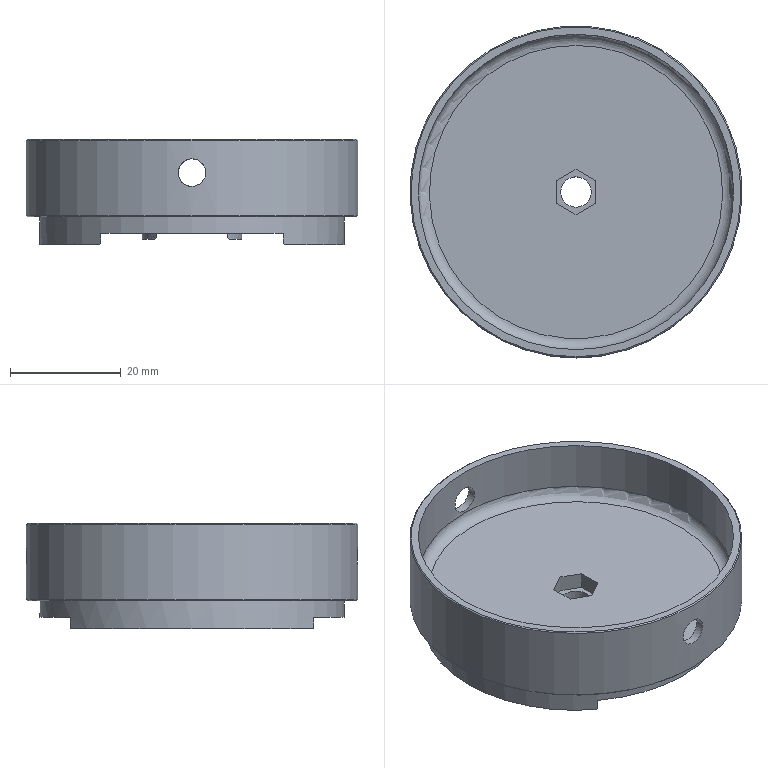NC program | NX | posted with a generic post | part box 60 x 60 x 19 mm
Lines 297 to 1274 of 13134:
(FLOOR_WALL_1_COPY_1 , TOOL : D17R0.8)
N586 T19 M6
N588 G54
N590 G17 G0 G90 X6.259 Y-4.944 S2000 M3
N592 G43 Z30. H19
N594 Z1.5
N596 G94 G1 X6.836 Y-4.214 Z1.451 F1000.
N598 X7.624 Y-2.522 Z1.353
N600 X8. Y-0.693 Z1.256
N602 Y0.693 Z1.183
N604 X7.624 Y2.522 Z1.085
N606 X6.836 Y4.214 Z0.987
N608 X5.678 Y5.678 Z0.889
N610 X4.214 Y6.836 Z0.792
N612 X2.522 Y7.624 Z0.694
N614 X0.693 Y8. Z0.596
N616 X-0.693 Z0.523
N618 X-2.522 Y7.624 Z0.425
N620 X-4.214 Y6.836 Z0.328
N622 X-5.678 Y5.678 Z0.23
N624 X-6.836 Y4.214 Z0.132
N626 X-7.624 Y2.522 Z0.034
N628 X-8. Y0.693 Z-0.064
N630 Y0. Z-0.1
N632 X-0.35
N634 G3 X0. Y-0.35 R0.35 F2000.
N636 X-0.35 Y0. R-0.35
N638 G1 X-8.
N640 G3 X0. Y-8. R8.
N642 X-8. Y0. R-8.
N644 G1 X-19.9
N646 G3 X0. Y-19.9 R19.9
N648 X-19.9 Y0. R-19.9
N650 G1 Z1.4
N652 G0 X-6.259 Y4.944
N654 G1 X-6.836 Y4.214 Z1.351 F1000.
N656 X-7.624 Y2.522 Z1.253
N658 X-8. Y0.693 Z1.156
N660 Y-0.693 Z1.083
N662 X-7.624 Y-2.522 Z0.985
N664 X-6.836 Y-4.214 Z0.887
N666 X-5.678 Y-5.678 Z0.789
N668 X-4.214 Y-6.836 Z0.692
N670 X-2.522 Y-7.624 Z0.594
N672 X-0.693 Y-8. Z0.496
N674 X0.693 Z0.423
N676 X2.522 Y-7.624 Z0.325
N678 X4.214 Y-6.836 Z0.228
N680 X5.678 Y-5.678 Z0.13
N682 X6.836 Y-4.214 Z0.032
N684 X7.624 Y-2.522 Z-0.066
N686 X8. Y-0.693 Z-0.164
N688 Y0. Z-0.2
N690 X0.35
N692 G3 X0. Y0.35 R0.35 F2000.
N694 X0.35 Y0. R-0.35
N696 G1 X8.
N698 G3 X0. Y8. R8.
N700 X8. Y0. R-8.
N702 G1 X19.9
N704 G3 X0. Y19.9 R19.9
N706 X19.9 Y0. R-19.9
N708 G1 Z1.3
N710 G0 X-6.259 Y4.944
N712 G1 X-6.836 Y4.214 Z1.251 F1000.
N714 X-7.624 Y2.522 Z1.153
N716 X-8. Y0.693 Z1.056
N718 Y-0.693 Z0.983
N720 X-7.624 Y-2.522 Z0.885
N722 X-6.836 Y-4.214 Z0.787
N724 X-5.678 Y-5.678 Z0.689
N726 X-4.214 Y-6.836 Z0.592
N728 X-2.522 Y-7.624 Z0.494
N730 X-0.693 Y-8. Z0.396
N732 X0.693 Z0.323
N734 X2.522 Y-7.624 Z0.225
N736 X4.214 Y-6.836 Z0.128
N738 X5.678 Y-5.678 Z0.03
N740 X6.836 Y-4.214 Z-0.068
N742 X7.624 Y-2.522 Z-0.166
N744 X8. Y-0.693 Z-0.264
N746 Y0. Z-0.3
N748 X0.35
N750 G3 X0. Y0.35 R0.35 F2000.
N752 X0.35 Y0. R-0.35
N754 G1 X8.
N756 G3 X0. Y8. R8.
N758 X8. Y0. R-8.
N760 G1 X19.9
N762 G3 X0. Y19.9 R19.9
N764 X19.9 Y0. R-19.9
N766 G1 Z1.2
N768 G0 X-6.259 Y4.944
N770 G1 X-6.836 Y4.214 Z1.151 F1000.
N772 X-7.624 Y2.522 Z1.053
N774 X-8. Y0.693 Z0.956
N776 Y-0.693 Z0.883
N778 X-7.624 Y-2.522 Z0.785
N780 X-6.836 Y-4.214 Z0.687
N782 X-5.678 Y-5.678 Z0.589
N784 X-4.214 Y-6.836 Z0.492
N786 X-2.522 Y-7.624 Z0.394
N788 X-0.693 Y-8. Z0.296
N790 X0.693 Z0.223
N792 X2.522 Y-7.624 Z0.125
N794 X4.214 Y-6.836 Z0.028
N796 X5.678 Y-5.678 Z-0.07
N798 X6.836 Y-4.214 Z-0.168
N800 X7.624 Y-2.522 Z-0.266
N802 X8. Y-0.693 Z-0.364
N804 Y0. Z-0.4
N806 X0.35
N808 G3 X0. Y0.35 R0.35 F2000.
N810 X0.35 Y0. R-0.35
N812 G1 X8.
N814 G3 X0. Y8. R8.
N816 X8. Y0. R-8.
N818 G1 X19.9
N820 G3 X0. Y19.9 R19.9
N822 X19.9 Y0. R-19.9
N824 G1 Z1.1
N826 G0 X-6.259 Y4.944
N828 G1 X-6.836 Y4.214 Z1.051 F1000.
N830 X-7.624 Y2.522 Z0.953
N832 X-8. Y0.693 Z0.856
N834 Y-0.693 Z0.783
N836 X-7.624 Y-2.522 Z0.685
N838 X-6.836 Y-4.214 Z0.587
N840 X-5.678 Y-5.678 Z0.489
N842 X-4.214 Y-6.836 Z0.392
N844 X-2.522 Y-7.624 Z0.294
N846 X-0.693 Y-8. Z0.196
N848 X0.693 Z0.123
N850 X2.522 Y-7.624 Z0.025
N852 X4.214 Y-6.836 Z-0.072
N854 X5.678 Y-5.678 Z-0.17
N856 X6.836 Y-4.214 Z-0.268
N858 X7.624 Y-2.522 Z-0.366
N860 X8. Y-0.693 Z-0.464
N862 Y0. Z-0.5
N864 X0.35
N866 G3 X0. Y0.35 R0.35 F2000.
N868 X0.35 Y0. R-0.35
N870 G1 X8.
N872 G3 X0. Y8. R8.
N874 X8. Y0. R-8.
N876 G1 X19.9
N878 G3 X0. Y19.9 R19.9
N880 X19.9 Y0. R-19.9
N882 G1 Z1.
N884 G0 X-6.259 Y4.944
N886 G1 X-6.836 Y4.214 Z0.951 F1000.
N888 X-7.624 Y2.522 Z0.853
N890 X-8. Y0.693 Z0.756
N892 Y-0.693 Z0.683
N894 X-7.624 Y-2.522 Z0.585
N896 X-6.836 Y-4.214 Z0.487
N898 X-5.678 Y-5.678 Z0.389
N900 X-4.214 Y-6.836 Z0.292
N902 X-2.522 Y-7.624 Z0.194
N904 X-0.693 Y-8. Z0.096
N906 X0.693 Z0.023
N908 X2.522 Y-7.624 Z-0.075
N910 X4.214 Y-6.836 Z-0.172
N912 X5.678 Y-5.678 Z-0.27
N914 X6.836 Y-4.214 Z-0.368
N916 X7.624 Y-2.522 Z-0.466
N918 X8. Y-0.693 Z-0.564
N920 Y0. Z-0.6
N922 X0.35
N924 G3 X0. Y0.35 R0.35 F2000.
N926 X0.35 Y0. R-0.35
N928 G1 X8.
N930 G3 X0. Y8. R8.
N932 X8. Y0. R-8.
N934 G1 X19.9
N936 G3 X0. Y19.9 R19.9
N938 X19.9 Y0. R-19.9
N940 G1 Z0.9
N942 G0 X-6.259 Y4.944
N944 G1 X-6.836 Y4.214 Z0.851 F1000.
N946 X-7.624 Y2.522 Z0.753
N948 X-8. Y0.693 Z0.656
N950 Y-0.693 Z0.583
N952 X-7.624 Y-2.522 Z0.485
N954 X-6.836 Y-4.214 Z0.387
N956 X-5.678 Y-5.678 Z0.289
N958 X-4.214 Y-6.836 Z0.192
N960 X-2.522 Y-7.624 Z0.094
N962 X-0.693 Y-8. Z-0.004
N964 X0.693 Z-0.077
N966 X2.522 Y-7.624 Z-0.175
N968 X4.214 Y-6.836 Z-0.272
N970 X5.678 Y-5.678 Z-0.37
N972 X6.836 Y-4.214 Z-0.468
N974 X7.624 Y-2.522 Z-0.566
N976 X8. Y-0.693 Z-0.664
N978 Y0. Z-0.7
N980 X0.35
N982 G3 X0. Y0.35 R0.35 F2000.
N984 X0.35 Y0. R-0.35
N986 G1 X8.
N988 G3 X0. Y8. R8.
N990 X8. Y0. R-8.
N992 G1 X19.9
N994 G3 X0. Y19.9 R19.9
N996 X19.9 Y0. R-19.9
N998 G1 Z0.8
N1000 G0 X-6.259 Y4.944
N1002 G1 X-6.836 Y4.214 Z0.751 F1000.
N1004 X-7.624 Y2.522 Z0.653
N1006 X-8. Y0.693 Z0.556
N1008 Y-0.693 Z0.483
N1010 X-7.624 Y-2.522 Z0.385
N1012 X-6.836 Y-4.214 Z0.287
N1014 X-5.678 Y-5.678 Z0.189
N1016 X-4.214 Y-6.836 Z0.092
N1018 X-2.522 Y-7.624 Z-0.006
N1020 X-0.693 Y-8. Z-0.104
N1022 X0.693 Z-0.177
N1024 X2.522 Y-7.624 Z-0.275
N1026 X4.214 Y-6.836 Z-0.372
N1028 X5.678 Y-5.678 Z-0.47
N1030 X6.836 Y-4.214 Z-0.568
N1032 X7.624 Y-2.522 Z-0.666
N1034 X8. Y-0.693 Z-0.764
N1036 Y0. Z-0.8
N1038 X0.35
N1040 G3 X0. Y0.35 R0.35 F2000.
N1042 X0.35 Y0. R-0.35
N1044 G1 X8.
N1046 G3 X0. Y8. R8.
N1048 X8. Y0. R-8.
N1050 G1 X19.9
N1052 G3 X0. Y19.9 R19.9
N1054 X19.9 Y0. R-19.9
N1056 G1 Z0.7
N1058 G0 X-6.259 Y4.944
N1060 G1 X-6.836 Y4.214 Z0.651 F1000.
N1062 X-7.624 Y2.522 Z0.553
N1064 X-8. Y0.693 Z0.456
N1066 Y-0.693 Z0.383
N1068 X-7.624 Y-2.522 Z0.285
N1070 X-6.836 Y-4.214 Z0.187
N1072 X-5.678 Y-5.678 Z0.089
N1074 X-4.214 Y-6.836 Z-0.008
N1076 X-2.522 Y-7.624 Z-0.106
N1078 X-0.693 Y-8. Z-0.204
N1080 X0.693 Z-0.277
N1082 X2.522 Y-7.624 Z-0.375
N1084 X4.214 Y-6.836 Z-0.472
N1086 X5.678 Y-5.678 Z-0.57
N1088 X6.836 Y-4.214 Z-0.668
N1090 X7.624 Y-2.522 Z-0.766
N1092 X8. Y-0.693 Z-0.864
N1094 Y0. Z-0.9
N1096 X0.35
N1098 G3 X0. Y0.35 R0.35 F2000.
N1100 X0.35 Y0. R-0.35
N1102 G1 X8.
N1104 G3 X0. Y8. R8.
N1106 X8. Y0. R-8.
N1108 G1 X19.9
N1110 G3 X0. Y19.9 R19.9
N1112 X19.9 Y0. R-19.9
N1114 G1 Z0.6
N1116 G0 X-6.259 Y4.944
N1118 G1 X-6.836 Y4.214 Z0.551 F1000.
N1120 X-7.624 Y2.522 Z0.453
N1122 X-8. Y0.693 Z0.356
N1124 Y-0.693 Z0.283
N1126 X-7.624 Y-2.522 Z0.185
N1128 X-6.836 Y-4.214 Z0.087
N1130 X-5.678 Y-5.678 Z-0.011
N1132 X-4.214 Y-6.836 Z-0.108
N1134 X-2.522 Y-7.624 Z-0.206
N1136 X-0.693 Y-8. Z-0.304
N1138 X0.693 Z-0.377
N1140 X2.522 Y-7.624 Z-0.475
N1142 X4.214 Y-6.836 Z-0.572
N1144 X5.678 Y-5.678 Z-0.67
N1146 X6.836 Y-4.214 Z-0.768
N1148 X7.624 Y-2.522 Z-0.866
N1150 X8. Y-0.693 Z-0.964
N1152 Y0. Z-1.
N1154 X0.35
N1156 G3 X0. Y0.35 R0.35 F2000.
N1158 X0.35 Y0. R-0.35
N1160 G1 X8.
N1162 G3 X0. Y8. R8.
N1164 X8. Y0. R-8.
N1166 G1 X19.9
N1168 G3 X0. Y19.9 R19.9
N1170 X19.9 Y0. R-19.9
N1172 G1 Z0.5
N1174 G0 X-6.259 Y4.944
N1176 G1 X-6.836 Y4.214 Z0.451 F1000.
N1178 X-7.624 Y2.522 Z0.353
N1180 X-8. Y0.693 Z0.256
N1182 Y-0.693 Z0.183
N1184 X-7.624 Y-2.522 Z0.085
N1186 X-6.836 Y-4.214 Z-0.013
N1188 X-5.678 Y-5.678 Z-0.111
N1190 X-4.214 Y-6.836 Z-0.208
N1192 X-2.522 Y-7.624 Z-0.306
N1194 X-0.693 Y-8. Z-0.404
N1196 X0.693 Z-0.477
N1198 X2.522 Y-7.624 Z-0.575
N1200 X4.214 Y-6.836 Z-0.672
N1202 X5.678 Y-5.678 Z-0.77
N1204 X6.836 Y-4.214 Z-0.868
N1206 X7.624 Y-2.522 Z-0.966
N1208 X8. Y-0.693 Z-1.064
N1210 Y0. Z-1.1
N1212 X0.35
N1214 G3 X0. Y0.35 R0.35 F2000.
N1216 X0.35 Y0. R-0.35
N1218 G1 X8.
N1220 G3 X0. Y8. R8.
N1222 X8. Y0. R-8.
N1224 G1 X19.9
N1226 G3 X0. Y19.9 R19.9
N1228 X19.9 Y0. R-19.9
N1230 G1 Z0.4
N1232 G0 X-6.259 Y4.944
N1234 G1 X-6.836 Y4.214 Z0.351 F1000.
N1236 X-7.624 Y2.522 Z0.253
N1238 X-8. Y0.693 Z0.156
N1240 Y-0.693 Z0.083
N1242 X-7.624 Y-2.522 Z-0.015
N1244 X-6.836 Y-4.214 Z-0.113
N1246 X-5.678 Y-5.678 Z-0.211
N1248 X-4.214 Y-6.836 Z-0.308
N1250 X-2.522 Y-7.624 Z-0.406
N1252 X-0.693 Y-8. Z-0.504
N1254 X0.693 Z-0.577
N1256 X2.522 Y-7.624 Z-0.675
N1258 X4.214 Y-6.836 Z-0.772
N1260 X5.678 Y-5.678 Z-0.87
N1262 X6.836 Y-4.214 Z-0.968
N1264 X7.624 Y-2.522 Z-1.066
N1266 X8. Y-0.693 Z-1.164
N1268 Y0. Z-1.2
N1270 X0.35
N1272 G3 X0. Y0.35 R0.35 F2000.
N1274 X0.35 Y0. R-0.35
N1276 G1 X8.
N1278 G3 X0. Y8. R8.
N1280 X8. Y0. R-8.
N1282 G1 X19.9
N1284 G3 X0. Y19.9 R19.9
N1286 X19.9 Y0. R-19.9
N1288 G1 Z0.3
N1290 G0 X-6.259 Y4.944
N1292 G1 X-6.836 Y4.214 Z0.251 F1000.
N1294 X-7.624 Y2.522 Z0.153
N1296 X-8. Y0.693 Z0.056
N1298 Y-0.693 Z-0.017
N1300 X-7.624 Y-2.522 Z-0.115
N1302 X-6.836 Y-4.214 Z-0.213
N1304 X-5.678 Y-5.678 Z-0.311
N1306 X-4.214 Y-6.836 Z-0.408
N1308 X-2.522 Y-7.624 Z-0.506
N1310 X-0.693 Y-8. Z-0.604
N1312 X0.693 Z-0.677
N1314 X2.522 Y-7.624 Z-0.775
N1316 X4.214 Y-6.836 Z-0.872
N1318 X5.678 Y-5.678 Z-0.97
N1320 X6.836 Y-4.214 Z-1.068
N1322 X7.624 Y-2.522 Z-1.166
N1324 X8. Y-0.693 Z-1.264
N1326 Y0. Z-1.3
N1328 X0.35
N1330 G3 X0. Y0.35 R0.35 F2000.
N1332 X0.35 Y0. R-0.35
N1334 G1 X8.
N1336 G3 X0. Y8. R8.
N1338 X8. Y0. R-8.
N1340 G1 X19.9
N1342 G3 X0. Y19.9 R19.9
N1344 X19.9 Y0. R-19.9
N1346 G1 Z0.2
N1348 G0 X-6.259 Y4.944
N1350 G1 X-6.836 Y4.214 Z0.151 F1000.
N1352 X-7.624 Y2.522 Z0.053
N1354 X-8. Y0.693 Z-0.044
N1356 Y-0.693 Z-0.117
N1358 X-7.624 Y-2.522 Z-0.215
N1360 X-6.836 Y-4.214 Z-0.313
N1362 X-5.678 Y-5.678 Z-0.411
N1364 X-4.214 Y-6.836 Z-0.508
N1366 X-2.522 Y-7.624 Z-0.606
N1368 X-0.693 Y-8. Z-0.704
N1370 X0.693 Z-0.777
N1372 X2.522 Y-7.624 Z-0.875
N1374 X4.214 Y-6.836 Z-0.972
N1376 X5.678 Y-5.678 Z-1.07
N1378 X6.836 Y-4.214 Z-1.168
N1380 X7.624 Y-2.522 Z-1.266
N1382 X8. Y-0.693 Z-1.364
N1384 Y0. Z-1.4
N1386 X0.35
N1388 G3 X0. Y0.35 R0.35 F2000.
N1390 X0.35 Y0. R-0.35
N1392 G1 X8.
N1394 G3 X0. Y8. R8.
N1396 X8. Y0. R-8.
N1398 G1 X19.9
N1400 G3 X0. Y19.9 R19.9
N1402 X19.9 Y0. R-19.9
N1404 G1 Z0.1
N1406 G0 X-6.259 Y4.944
N1408 G1 X-6.836 Y4.214 Z0.051 F1000.
N1410 X-7.624 Y2.522 Z-0.047
N1412 X-8. Y0.693 Z-0.144
N1414 Y-0.693 Z-0.217
N1416 X-7.624 Y-2.522 Z-0.315
N1418 X-6.836 Y-4.214 Z-0.413
N1420 X-5.678 Y-5.678 Z-0.511
N1422 X-4.214 Y-6.836 Z-0.608
N1424 X-2.522 Y-7.624 Z-0.706
N1426 X-0.693 Y-8. Z-0.804
N1428 X0.693 Z-0.877
N1430 X2.522 Y-7.624 Z-0.975
N1432 X4.214 Y-6.836 Z-1.072
N1434 X5.678 Y-5.678 Z-1.17
N1436 X6.836 Y-4.214 Z-1.268
N1438 X7.624 Y-2.522 Z-1.366
N1440 X8. Y-0.693 Z-1.464
N1442 Y0. Z-1.5
N1444 X0.35
N1446 G3 X0. Y0.35 R0.35 F2000.
N1448 X0.35 Y0. R-0.35
N1450 G1 X8.
N1452 G3 X0. Y8. R8.
N1454 X8. Y0. R-8.
N1456 G1 X19.9
N1458 G3 X0. Y19.9 R19.9
N1460 X19.9 Y0. R-19.9
N1462 G1 Z0.
N1464 G0 X-6.259 Y4.944
N1466 G1 X-6.836 Y4.214 Z-0.049 F1000.
N1468 X-7.624 Y2.522 Z-0.147
N1470 X-8. Y0.693 Z-0.244
N1472 Y-0.693 Z-0.317
N1474 X-7.624 Y-2.522 Z-0.415
N1476 X-6.836 Y-4.214 Z-0.513
N1478 X-5.678 Y-5.678 Z-0.611
N1480 X-4.214 Y-6.836 Z-0.708
N1482 X-2.522 Y-7.624 Z-0.806
N1484 X-0.693 Y-8. Z-0.904
N1486 X0.693 Z-0.977
N1488 X2.522 Y-7.624 Z-1.075
N1490 X4.214 Y-6.836 Z-1.172
N1492 X5.678 Y-5.678 Z-1.27
N1494 X6.836 Y-4.214 Z-1.368
N1496 X7.624 Y-2.522 Z-1.466
N1498 X8. Y-0.693 Z-1.564
N1500 Y0. Z-1.6
N1502 X0.35
N1504 G3 X0. Y0.35 R0.35 F2000.
N1506 X0.35 Y0. R-0.35
N1508 G1 X8.
N1510 G3 X0. Y8. R8.
N1512 X8. Y0. R-8.
N1514 G1 X19.9
N1516 G3 X0. Y19.9 R19.9
N1518 X19.9 Y0. R-19.9
N1520 G1 Z-0.1
N1522 G0 X-6.259 Y4.944
N1524 G1 X-6.836 Y4.214 Z-0.149 F1000.
N1526 X-7.624 Y2.522 Z-0.247
N1528 X-8. Y0.693 Z-0.344
N1530 Y-0.693 Z-0.417
N1532 X-7.624 Y-2.522 Z-0.515
N1534 X-6.836 Y-4.214 Z-0.613
N1536 X-5.678 Y-5.678 Z-0.711
N1538 X-4.214 Y-6.836 Z-0.808
N1540 X-2.522 Y-7.624 Z-0.906
N1542 X-0.693 Y-8. Z-1.004
N1544 X0.693 Z-1.077
N1546 X2.522 Y-7.624 Z-1.175
N1548 X4.214 Y-6.836 Z-1.272
N1550 X5.678 Y-5.678 Z-1.37
N1552 X6.836 Y-4.214 Z-1.468
N1554 X7.624 Y-2.522 Z-1.566
N1556 X8. Y-0.693 Z-1.664
N1558 Y0. Z-1.7
N1560 X0.35
N1562 G3 X0. Y0.35 R0.35 F2000.
N1564 X0.35 Y0. R-0.35
N1566 G1 X8.
N1568 G3 X0. Y8. R8.
N1570 X8. Y0. R-8.
N1572 G1 X19.9
N1574 G3 X0. Y19.9 R19.9
N1576 X19.9 Y0. R-19.9
N1578 G1 Z-0.2
N1580 G0 X-6.259 Y4.944
N1582 G1 X-6.836 Y4.214 Z-0.249 F1000.
N1584 X-7.624 Y2.522 Z-0.347
N1586 X-8. Y0.693 Z-0.444
N1588 Y-0.693 Z-0.517
N1590 X-7.624 Y-2.522 Z-0.615
N1592 X-6.836 Y-4.214 Z-0.713
N1594 X-5.678 Y-5.678 Z-0.811
N1596 X-4.214 Y-6.836 Z-0.908
N1598 X-2.522 Y-7.624 Z-1.006
N1600 X-0.693 Y-8. Z-1.104
N1602 X0.693 Z-1.177
N1604 X2.522 Y-7.624 Z-1.275
N1606 X4.214 Y-6.836 Z-1.372
N1608 X5.678 Y-5.678 Z-1.47
N1610 X6.836 Y-4.214 Z-1.568
N1612 X7.624 Y-2.522 Z-1.666
N1614 X8. Y-0.693 Z-1.764
N1616 Y0. Z-1.8
N1618 X0.35
N1620 G3 X0. Y0.35 R0.35 F2000.
N1622 X0.35 Y0. R-0.35
N1624 G1 X8.
N1626 G3 X0. Y8. R8.
N1628 X8. Y0. R-8.
N1630 G1 X19.9
N1632 G3 X0. Y19.9 R19.9
N1634 X19.9 Y0. R-19.9
N1636 G1 Z-0.3
N1638 G0 X-6.259 Y4.944
N1640 G1 X-6.836 Y4.214 Z-0.349 F1000.
N1642 X-7.624 Y2.522 Z-0.447
N1644 X-8. Y0.693 Z-0.544
N1646 Y-0.693 Z-0.617
N1648 X-7.624 Y-2.522 Z-0.715
N1650 X-6.836 Y-4.214 Z-0.813
N1652 X-5.678 Y-5.678 Z-0.911
N1654 X-4.214 Y-6.836 Z-1.008
N1656 X-2.522 Y-7.624 Z-1.106
N1658 X-0.693 Y-8. Z-1.204
N1660 X0.693 Z-1.277
N1662 X2.522 Y-7.624 Z-1.375
N1664 X4.214 Y-6.836 Z-1.472
N1666 X5.678 Y-5.678 Z-1.57
N1668 X6.836 Y-4.214 Z-1.668
N1670 X7.624 Y-2.522 Z-1.766
N1672 X8. Y-0.693 Z-1.864
N1674 Y0. Z-1.9
N1676 X0.35
N1678 G3 X0. Y0.35 R0.35 F2000.
N1680 X0.35 Y0. R-0.35
N1682 G1 X8.
N1684 G3 X0. Y8. R8.
N1686 X8. Y0. R-8.
N1688 G1 X19.9
N1690 G3 X0. Y19.9 R19.9
N1692 X19.9 Y0. R-19.9
N1694 G1 Z-0.4
N1696 G0 X-6.259 Y4.944
N1698 G1 X-6.836 Y4.214 Z-0.449 F1000.
N1700 X-7.624 Y2.522 Z-0.547
N1702 X-8. Y0.693 Z-0.644
N1704 Y-0.693 Z-0.717
N1706 X-7.624 Y-2.522 Z-0.815
N1708 X-6.836 Y-4.214 Z-0.913
N1710 X-5.678 Y-5.678 Z-1.011
N1712 X-4.214 Y-6.836 Z-1.108
N1714 X-2.522 Y-7.624 Z-1.206
N1716 X-0.693 Y-8. Z-1.304
N1718 X0.693 Z-1.377
N1720 X2.522 Y-7.624 Z-1.475
N1722 X4.214 Y-6.836 Z-1.572
N1724 X5.678 Y-5.678 Z-1.67
N1726 X6.836 Y-4.214 Z-1.768
N1728 X7.624 Y-2.522 Z-1.866
N1730 X8. Y-0.693 Z-1.964
N1732 Y0. Z-2.
N1734 X0.35
N1736 G3 X0. Y0.35 R0.35 F2000.
N1738 X0.35 Y0. R-0.35
N1740 G1 X8.
N1742 G3 X0. Y8. R8.
N1744 X8. Y0. R-8.
N1746 G1 X19.9
N1748 G3 X0. Y19.9 R19.9
N1750 X19.9 Y0. R-19.9
N1752 G1 Z-0.5
N1754 G0 X-6.259 Y4.944
N1756 G1 X-6.836 Y4.214 Z-0.549 F1000.
N1758 X-7.624 Y2.522 Z-0.647
N1760 X-8. Y0.693 Z-0.744
N1762 Y-0.693 Z-0.817
N1764 X-7.624 Y-2.522 Z-0.915
N1766 X-6.836 Y-4.214 Z-1.013
N1768 X-5.678 Y-5.678 Z-1.111
N1770 X-4.214 Y-6.836 Z-1.208
N1772 X-2.522 Y-7.624 Z-1.306
N1774 X-0.693 Y-8. Z-1.404
N1776 X0.693 Z-1.477
N1778 X2.522 Y-7.624 Z-1.575
N1780 X4.214 Y-6.836 Z-1.672
N1782 X5.678 Y-5.678 Z-1.77
N1784 X6.836 Y-4.214 Z-1.868
N1786 X7.624 Y-2.522 Z-1.966
N1788 X8. Y-0.693 Z-2.064
N1790 Y0. Z-2.1
N1792 X0.35
N1794 G3 X0. Y0.35 R0.35 F2000.
N1796 X0.35 Y0. R-0.35
N1798 G1 X8.
N1800 G3 X0. Y8. R8.
N1802 X8. Y0. R-8.
N1804 G1 X19.9
N1806 G3 X0. Y19.9 R19.9
N1808 X19.9 Y0. R-19.9
N1810 G1 Z-0.6
N1812 G0 X-6.259 Y4.944
N1814 G1 X-6.836 Y4.214 Z-0.649 F1000.
N1816 X-7.624 Y2.522 Z-0.747
N1818 X-8. Y0.693 Z-0.844
N1820 Y-0.693 Z-0.917
N1822 X-7.624 Y-2.522 Z-1.015
N1824 X-6.836 Y-4.214 Z-1.113
N1826 X-5.678 Y-5.678 Z-1.211
N1828 X-4.214 Y-6.836 Z-1.308
N1830 X-2.522 Y-7.624 Z-1.406
N1832 X-0.693 Y-8. Z-1.504
N1834 X0.693 Z-1.577
N1836 X2.522 Y-7.624 Z-1.675
N1838 X4.214 Y-6.836 Z-1.772
N1840 X5.678 Y-5.678 Z-1.87
N1842 X6.836 Y-4.214 Z-1.968
N1844 X7.624 Y-2.522 Z-2.066
N1846 X8. Y-0.693 Z-2.164
N1848 Y0. Z-2.2
N1850 X0.35
N1852 G3 X0. Y0.35 R0.35 F2000.
N1854 X0.35 Y0. R-0.35
N1856 G1 X8.
N1858 G3 X0. Y8. R8.
N1860 X8. Y0. R-8.
N1862 G1 X19.9
N1864 G3 X0. Y19.9 R19.9
N1866 X19.9 Y0. R-19.9
N1868 G1 Z-0.7
N1870 G0 X-6.259 Y4.944
N1872 G1 X-6.836 Y4.214 Z-0.749 F1000.
N1874 X-7.624 Y2.522 Z-0.847
N1876 X-8. Y0.693 Z-0.944
N1878 Y-0.693 Z-1.017
N1880 X-7.624 Y-2.522 Z-1.115
N1882 X-6.836 Y-4.214 Z-1.213
N1884 X-5.678 Y-5.678 Z-1.311
N1886 X-4.214 Y-6.836 Z-1.408
N1888 X-2.522 Y-7.624 Z-1.506
N1890 X-0.693 Y-8. Z-1.604
N1892 X0.693 Z-1.677
N1894 X2.522 Y-7.624 Z-1.775
N1896 X4.214 Y-6.836 Z-1.872
N1898 X5.678 Y-5.678 Z-1.97
N1900 X6.836 Y-4.214 Z-2.068
N1902 X7.624 Y-2.522 Z-2.166
N1904 X8. Y-0.693 Z-2.264
N1906 Y0. Z-2.3
N1908 X0.35
N1910 G3 X0. Y0.35 R0.35 F2000.
N1912 X0.35 Y0. R-0.35
N1914 G1 X8.
N1916 G3 X0. Y8. R8.
N1918 X8. Y0. R-8.
N1920 G1 X19.9
N1922 G3 X0. Y19.9 R19.9
N1924 X19.9 Y0. R-19.9
N1926 G1 Z-0.8
N1928 G0 X-6.259 Y4.944
N1930 G1 X-6.836 Y4.214 Z-0.849 F1000.
N1932 X-7.624 Y2.522 Z-0.947
N1934 X-8. Y0.693 Z-1.044
N1936 Y-0.693 Z-1.117
N1938 X-7.624 Y-2.522 Z-1.215
N1940 X-6.836 Y-4.214 Z-1.313
N1942 X-5.678 Y-5.678 Z-1.411
N1944 X-4.214 Y-6.836 Z-1.508
N1946 X-2.522 Y-7.624 Z-1.606
N1948 X-0.693 Y-8. Z-1.704
N1950 X0.693 Z-1.777
N1952 X2.522 Y-7.624 Z-1.875
N1954 X4.214 Y-6.836 Z-1.972
N1956 X5.678 Y-5.678 Z-2.07
N1958 X6.836 Y-4.214 Z-2.168
N1960 X7.624 Y-2.522 Z-2.266
N1962 X8. Y-0.693 Z-2.364
N1964 Y0. Z-2.4
N1966 X0.35
N1968 G3 X0. Y0.35 R0.35 F2000.
N1970 X0.35 Y0. R-0.35
N1972 G1 X8.
N1974 G3 X0. Y8. R8.
N1976 X8. Y0. R-8.
N1978 G1 X19.9
N1980 G3 X0. Y19.9 R19.9
N1982 X19.9 Y0. R-19.9
N1984 G1 Z-0.9
N1986 G0 X-6.259 Y4.944
N1988 G1 X-6.836 Y4.214 Z-0.949 F1000.
N1990 X-7.624 Y2.522 Z-1.047
N1992 X-8. Y0.693 Z-1.144
N1994 Y-0.693 Z-1.217
N1996 X-7.624 Y-2.522 Z-1.315
N1998 X-6.836 Y-4.214 Z-1.413
N2000 X-5.678 Y-5.678 Z-1.511
N2002 X-4.214 Y-6.836 Z-1.608
N2004 X-2.522 Y-7.624 Z-1.706
N2006 X-0.693 Y-8. Z-1.804
N2008 X0.693 Z-1.877
N2010 X2.522 Y-7.624 Z-1.975
N2012 X4.214 Y-6.836 Z-2.072
N2014 X5.678 Y-5.678 Z-2.17
N2016 X6.836 Y-4.214 Z-2.268
N2018 X7.624 Y-2.522 Z-2.366
N2020 X8. Y-0.693 Z-2.464
N2022 Y0. Z-2.5
N2024 X0.35
N2026 G3 X0. Y0.35 R0.35 F2000.
N2028 X0.35 Y0. R-0.35
N2030 G1 X8.
N2032 G3 X0. Y8. R8.
N2034 X8. Y0. R-8.
N2036 G1 X19.9
N2038 G3 X0. Y19.9 R19.9
N2040 X19.9 Y0. R-19.9
N2042 G1 Z-1.
N2044 G0 X-6.259 Y4.944
N2046 G1 X-6.836 Y4.214 Z-1.049 F1000.
N2048 X-7.624 Y2.522 Z-1.147
N2050 X-8. Y0.693 Z-1.244
N2052 Y-0.693 Z-1.317
N2054 X-7.624 Y-2.522 Z-1.415
N2056 X-6.836 Y-4.214 Z-1.513
N2058 X-5.678 Y-5.678 Z-1.611
N2060 X-4.214 Y-6.836 Z-1.708
N2062 X-2.522 Y-7.624 Z-1.806
N2064 X-0.693 Y-8. Z-1.904
N2066 X0.693 Z-1.977
N2068 X2.522 Y-7.624 Z-2.075
N2070 X4.214 Y-6.836 Z-2.172
N2072 X5.678 Y-5.678 Z-2.27
N2074 X6.836 Y-4.214 Z-2.368
N2076 X7.624 Y-2.522 Z-2.466
N2078 X8. Y-0.693 Z-2.564
N2080 Y0. Z-2.6
N2082 X0.35
N2084 G3 X0. Y0.35 R0.35 F2000.
N2086 X0.35 Y0. R-0.35
N2088 G1 X8.
N2090 G3 X0. Y8. R8.
N2092 X8. Y0. R-8.
N2094 G1 X19.9
N2096 G3 X0. Y19.9 R19.9
N2098 X19.9 Y0. R-19.9
N2100 G1 Z-1.1
N2102 G0 X-6.259 Y4.944
N2104 G1 X-6.836 Y4.214 Z-1.149 F1000.
N2106 X-7.624 Y2.522 Z-1.247
N2108 X-8. Y0.693 Z-1.344
N2110 Y-0.693 Z-1.417
N2112 X-7.624 Y-2.522 Z-1.515
N2114 X-6.836 Y-4.214 Z-1.613
N2116 X-5.678 Y-5.678 Z-1.711
N2118 X-4.214 Y-6.836 Z-1.808
N2120 X-2.522 Y-7.624 Z-1.906
N2122 X-0.693 Y-8. Z-2.004
N2124 X0.693 Z-2.077
N2126 X2.522 Y-7.624 Z-2.175
N2128 X4.214 Y-6.836 Z-2.272
N2130 X5.678 Y-5.678 Z-2.37
N2132 X6.836 Y-4.214 Z-2.468
N2134 X7.624 Y-2.522 Z-2.566
N2136 X8. Y-0.693 Z-2.664
N2138 Y0. Z-2.7
N2140 X0.35
N2142 G3 X0. Y0.35 R0.35 F2000.
N2144 X0.35 Y0. R-0.35
N2146 G1 X8.
N2148 G3 X0. Y8. R8.
N2150 X8. Y0. R-8.
N2152 G1 X19.9
N2154 G3 X0. Y19.9 R19.9
N2156 X19.9 Y0. R-19.9
N2158 G1 Z-1.2
N2160 G0 X-6.259 Y4.944
N2162 G1 X-6.836 Y4.214 Z-1.249 F1000.
N2164 X-7.624 Y2.522 Z-1.347
N2166 X-8. Y0.693 Z-1.444
N2168 Y-0.693 Z-1.517
N2170 X-7.624 Y-2.522 Z-1.615
N2172 X-6.836 Y-4.214 Z-1.713
N2174 X-5.678 Y-5.678 Z-1.811
N2176 X-4.214 Y-6.836 Z-1.908
N2178 X-2.522 Y-7.624 Z-2.006
N2180 X-0.693 Y-8. Z-2.104
N2182 X0.693 Z-2.177
N2184 X2.522 Y-7.624 Z-2.275
N2186 X4.214 Y-6.836 Z-2.372
N2188 X5.678 Y-5.678 Z-2.47
N2190 X6.836 Y-4.214 Z-2.568
N2192 X7.624 Y-2.522 Z-2.666
N2194 X8. Y-0.693 Z-2.764
N2196 Y0. Z-2.8
N2198 X0.35
N2200 G3 X0. Y0.35 R0.35 F2000.
N2202 X0.35 Y0. R-0.35
N2204 G1 X8.
N2206 G3 X0. Y8. R8.
N2208 X8. Y0. R-8.
N2210 G1 X19.9
N2212 G3 X0. Y19.9 R19.9
N2214 X19.9 Y0. R-19.9
N2216 G1 Z-1.3
N2218 G0 X-6.259 Y4.944
N2220 G1 X-6.836 Y4.214 Z-1.349 F1000.
N2222 X-7.624 Y2.522 Z-1.447
N2224 X-8. Y0.693 Z-1.544
N2226 Y-0.693 Z-1.617
N2228 X-7.624 Y-2.522 Z-1.715
N2230 X-6.836 Y-4.214 Z-1.813
N2232 X-5.678 Y-5.678 Z-1.911
N2234 X-4.214 Y-6.836 Z-2.008
N2236 X-2.522 Y-7.624 Z-2.106
N2238 X-0.693 Y-8. Z-2.204
N2240 X0.693 Z-2.277
N2242 X2.522 Y-7.624 Z-2.375
N2244 X4.214 Y-6.836 Z-2.472
N2246 X5.678 Y-5.678 Z-2.57
N2248 X6.836 Y-4.214 Z-2.668
N2250 X7.624 Y-2.522 Z-2.766
N2252 X8. Y-0.693 Z-2.864
N2254 Y0. Z-2.9
N2256 X0.35
N2258 G3 X0. Y0.35 R0.35 F2000.
N2260 X0.35 Y0. R-0.35
N2262 G1 X8.
N2264 G3 X0. Y8. R8.
N2266 X8. Y0. R-8.
N2268 G1 X19.9
N2270 G3 X0. Y19.9 R19.9
N2272 X19.9 Y0. R-19.9
N2274 G1 Z-1.4
N2276 G0 X-6.259 Y4.944
N2278 G1 X-6.836 Y4.214 Z-1.449 F1000.
N2280 X-7.624 Y2.522 Z-1.547
N2282 X-8. Y0.693 Z-1.644
N2284 Y-0.693 Z-1.717
N2286 X-7.624 Y-2.522 Z-1.815
N2288 X-6.836 Y-4.214 Z-1.913
N2290 X-5.678 Y-5.678 Z-2.011
N2292 X-4.214 Y-6.836 Z-2.108
N2294 X-2.522 Y-7.624 Z-2.206
N2296 X-0.693 Y-8. Z-2.304
N2298 X0.693 Z-2.377
N2300 X2.522 Y-7.624 Z-2.475
N2302 X4.214 Y-6.836 Z-2.572
N2304 X5.678 Y-5.678 Z-2.67
N2306 X6.836 Y-4.214 Z-2.768
N2308 X7.624 Y-2.522 Z-2.866
N2310 X8. Y-0.693 Z-2.964
N2312 Y0. Z-3.
N2314 X0.35
N2316 G3 X0. Y0.35 R0.35 F2000.
N2318 X0.35 Y0. R-0.35
N2320 G1 X8.
N2322 G3 X0. Y8. R8.
N2324 X8. Y0. R-8.
N2326 G1 X19.9
N2328 G3 X0. Y19.9 R19.9
N2330 X19.9 Y0. R-19.9
N2332 G1 Z-1.5
N2334 G0 X-6.259 Y4.944
N2336 G1 X-6.836 Y4.214 Z-1.549 F1000.
N2338 X-7.624 Y2.522 Z-1.647
N2340 X-8. Y0.693 Z-1.744
N2342 Y-0.693 Z-1.817
N2344 X-7.624 Y-2.522 Z-1.915
N2346 X-6.836 Y-4.214 Z-2.013
N2348 X-5.678 Y-5.678 Z-2.111
N2350 X-4.214 Y-6.836 Z-2.208
N2352 X-2.522 Y-7.624 Z-2.306
N2354 X-0.693 Y-8. Z-2.404
N2356 X0.693 Z-2.477
N2358 X2.522 Y-7.624 Z-2.575
N2360 X4.214 Y-6.836 Z-2.672
N2362 X5.678 Y-5.678 Z-2.77
N2364 X6.836 Y-4.214 Z-2.868
N2366 X7.624 Y-2.522 Z-2.966
N2368 X8. Y-0.693 Z-3.064
N2370 Y0. Z-3.1
N2372 X0.35
N2374 G3 X0. Y0.35 R0.35 F2000.
N2376 X0.35 Y0. R-0.35
N2378 G1 X8.
N2380 G3 X0. Y8. R8.
N2382 X8. Y0. R-8.
N2384 G1 X19.9
N2386 G3 X0. Y19.9 R19.9
N2388 X19.9 Y0. R-19.9
N2390 G1 Z-1.6
N2392 G0 X-6.259 Y4.944
N2394 G1 X-6.836 Y4.214 Z-1.649 F1000.
N2396 X-7.624 Y2.522 Z-1.747
N2398 X-8. Y0.693 Z-1.844
N2400 Y-0.693 Z-1.917
N2402 X-7.624 Y-2.522 Z-2.015
N2404 X-6.836 Y-4.214 Z-2.113
N2406 X-5.678 Y-5.678 Z-2.211
N2408 X-4.214 Y-6.836 Z-2.308
N2410 X-2.522 Y-7.624 Z-2.406
N2412 X-0.693 Y-8. Z-2.504
N2414 X0.693 Z-2.577
N2416 X2.522 Y-7.624 Z-2.675
N2418 X4.214 Y-6.836 Z-2.772
N2420 X5.678 Y-5.678 Z-2.87
N2422 X6.836 Y-4.214 Z-2.968
N2424 X7.624 Y-2.522 Z-3.066
N2426 X8. Y-0.693 Z-3.164
N2428 Y0. Z-3.2
N2430 X0.35
N2432 G3 X0. Y0.35 R0.35 F2000.
N2434 X0.35 Y0. R-0.35
N2436 G1 X8.
N2438 G3 X0. Y8. R8.
N2440 X8. Y0. R-8.
N2442 G1 X19.9
N2444 G3 X0. Y19.9 R19.9
N2446 X19.9 Y0. R-19.9
N2448 G1 Z-1.7
N2450 G0 X-6.259 Y4.944
N2452 G1 X-6.836 Y4.214 Z-1.749 F1000.
N2454 X-7.624 Y2.522 Z-1.847
N2456 X-8. Y0.693 Z-1.944
N2458 Y-0.693 Z-2.017
N2460 X-7.624 Y-2.522 Z-2.115
N2462 X-6.836 Y-4.214 Z-2.213
N2464 X-5.678 Y-5.678 Z-2.311
N2466 X-4.214 Y-6.836 Z-2.408
N2468 X-2.522 Y-7.624 Z-2.506
N2470 X-0.693 Y-8. Z-2.604
N2472 X0.693 Z-2.677
N2474 X2.522 Y-7.624 Z-2.775
N2476 X4.214 Y-6.836 Z-2.872
N2478 X5.678 Y-5.678 Z-2.97
N2480 X6.836 Y-4.214 Z-3.068
N2482 X7.624 Y-2.522 Z-3.166
N2484 X8. Y-0.693 Z-3.264
N2486 Y0. Z-3.3
N2488 X0.35
N2490 G3 X0. Y0.35 R0.35 F2000.
N2492 X0.35 Y0. R-0.35
N2494 G1 X8.
N2496 G3 X0. Y8. R8.
N2498 X8. Y0. R-8.
N2500 G1 X19.9
N2502 G3 X0. Y19.9 R19.9
N2504 X19.9 Y0. R-19.9
N2506 G1 Z-1.8
N2508 G0 X-6.259 Y4.944
N2510 G1 X-6.836 Y4.214 Z-1.849 F1000.
N2512 X-7.624 Y2.522 Z-1.947
N2514 X-8. Y0.693 Z-2.044
N2516 Y-0.693 Z-2.117
N2518 X-7.624 Y-2.522 Z-2.215
N2520 X-6.836 Y-4.214 Z-2.313
N2522 X-5.678 Y-5.678 Z-2.411
N2524 X-4.214 Y-6.836 Z-2.508
N2526 X-2.522 Y-7.624 Z-2.606
N2528 X-0.693 Y-8. Z-2.704
N2530 X0.693 Z-2.777
N2532 X2.522 Y-7.624 Z-2.875
N2534 X4.214 Y-6.836 Z-2.972